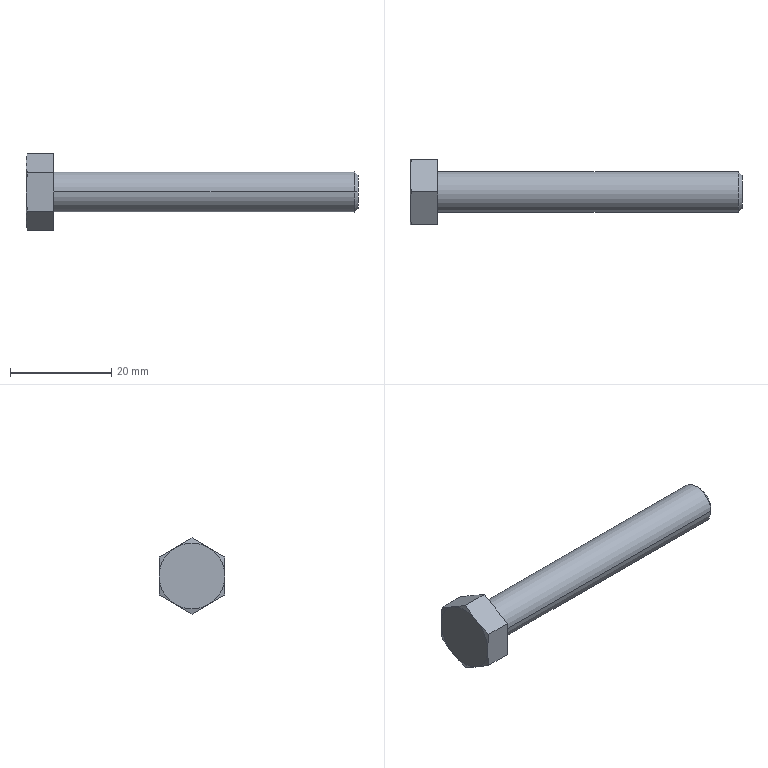Part | STEP file | TNSN20-Y20-F22-Part-1-1 | 1 solid | 19 faces | box 65.5 x 13.002 x 15.011 mm | volume 3813 mm3 | plane 9 | cone 8 | cylinder 2 | commonest cylinder face diameters 8 x2
STEP:
#1=CARTESIAN_POINT('',(13990.745,13720.046,26.506));
#2=VERTEX_POINT('',#1);
#3=CARTESIAN_POINT('',(13990.745,13713.546,22.753));
#4=VERTEX_POINT('',#3);
#5=CARTESIAN_POINT('',(13990.745,13720.046,26.506));
#6=DIRECTION('',(0.,-0.866,-0.5));
#7=VECTOR('',#6,1000.);
#8=LINE('',#5,#7);
#9=EDGE_CURVE('',#2,#4,#8,.T.);
#10=ORIENTED_EDGE('',*,*,#9,.T.);
#11=CARTESIAN_POINT('',(13990.745,13713.546,15.247));
#12=VERTEX_POINT('',#11);
#13=CARTESIAN_POINT('',(13990.745,13713.546,22.753));
#14=DIRECTION('',(0.,0.,-1.));
#15=VECTOR('',#14,1000.);
#16=LINE('',#13,#15);
#17=EDGE_CURVE('',#4,#12,#16,.T.);
#18=ORIENTED_EDGE('',*,*,#17,.T.);
#19=CARTESIAN_POINT('',(13990.745,13720.046,11.494));
#20=VERTEX_POINT('',#19);
#21=CARTESIAN_POINT('',(13990.745,13713.546,15.247));
#22=DIRECTION('',(0.,0.866,-0.5));
#23=VECTOR('',#22,1000.);
#24=LINE('',#21,#23);
#25=EDGE_CURVE('',#12,#20,#24,.T.);
#26=ORIENTED_EDGE('',*,*,#25,.T.);
#27=CARTESIAN_POINT('',(13990.745,13726.546,15.247));
#28=VERTEX_POINT('',#27);
#29=CARTESIAN_POINT('',(13990.745,13720.046,11.494));
#30=DIRECTION('',(0.,0.866,0.5));
#31=VECTOR('',#30,1000.);
#32=LINE('',#29,#31);
#33=EDGE_CURVE('',#20,#28,#32,.T.);
#34=ORIENTED_EDGE('',*,*,#33,.T.);
#35=CARTESIAN_POINT('',(13990.745,13726.546,22.753));
#36=VERTEX_POINT('',#35);
#37=CARTESIAN_POINT('',(13990.745,13726.546,15.247));
#38=DIRECTION('',(0.,0.,1.));
#39=VECTOR('',#38,1000.);
#40=LINE('',#37,#39);
#41=EDGE_CURVE('',#28,#36,#40,.T.);
#42=ORIENTED_EDGE('',*,*,#41,.T.);
#43=CARTESIAN_POINT('',(13990.745,13726.546,22.753));
#44=DIRECTION('',(0.,-0.866,0.5));
#45=VECTOR('',#44,1000.);
#46=LINE('',#43,#45);
#47=EDGE_CURVE('',#36,#2,#46,.T.);
#48=ORIENTED_EDGE('',*,*,#47,.T.);
#49=EDGE_LOOP('',(#10,#18,#26,#34,#42,#48));
#50=FACE_OUTER_BOUND('',#49,.T.);
#51=CARTESIAN_POINT('',(13990.745,13716.046,19.));
#52=VERTEX_POINT('',#51);
#53=CARTESIAN_POINT('',(13990.745,13724.046,19.));
#54=VERTEX_POINT('',#53);
#55=CARTESIAN_POINT('',(13990.745,13720.046,19.));
#56=DIRECTION('',(1.,0.,0.));
#57=DIRECTION('',(0.,1.,0.));
#58=AXIS2_PLACEMENT_3D('',#55,#56,#57);
#59=CIRCLE('',#58,4.);
#60=EDGE_CURVE('',#52,#54,#59,.T.);
#61=ORIENTED_EDGE('',*,*,#60,.F.);
#62=CARTESIAN_POINT('',(13990.745,13720.046,19.));
#63=DIRECTION('',(1.,0.,0.));
#64=DIRECTION('',(0.,1.,0.));
#65=AXIS2_PLACEMENT_3D('',#62,#63,#64);
#66=CIRCLE('',#65,4.);
#67=EDGE_CURVE('',#54,#52,#66,.T.);
#68=ORIENTED_EDGE('',*,*,#67,.F.);
#69=EDGE_LOOP('',(#61,#68));
#70=FACE_BOUND('',#69,.T.);
#71=CARTESIAN_POINT('',(13990.745,13734.949,3.347));
#72=DIRECTION('',(-1.,0.,0.));
#73=DIRECTION('',(0.,-1.,0.));
#74=AXIS2_PLACEMENT_3D('',#71,#72,#73);
#75=PLANE('',#74);
#76=ADVANCED_FACE('',(#50,#70),#75,.F.);
#77=CARTESIAN_POINT('',(14050.745,13723.279,19.));
#78=VERTEX_POINT('',#77);
#79=CARTESIAN_POINT('',(14050.745,13716.813,19.));
#80=VERTEX_POINT('',#79);
#81=CARTESIAN_POINT('',(14050.745,13720.046,19.));
#82=DIRECTION('',(1.,0.,0.));
#83=DIRECTION('',(0.,1.,0.));
#84=AXIS2_PLACEMENT_3D('',#81,#82,#83);
#85=CIRCLE('',#84,3.233);
#86=EDGE_CURVE('',#78,#80,#85,.T.);
#87=ORIENTED_EDGE('',*,*,#86,.T.);
#88=CARTESIAN_POINT('',(14050.745,13720.046,19.));
#89=DIRECTION('',(1.,0.,0.));
#90=DIRECTION('',(0.,1.,0.));
#91=AXIS2_PLACEMENT_3D('',#88,#89,#90);
#92=CIRCLE('',#91,3.233);
#93=EDGE_CURVE('',#80,#78,#92,.T.);
#94=ORIENTED_EDGE('',*,*,#93,.T.);
#95=EDGE_LOOP('',(#87,#94));
#96=FACE_OUTER_BOUND('',#95,.T.);
#97=CARTESIAN_POINT('',(14050.745,13729.541,7.888));
#98=DIRECTION('',(-1.,0.,0.));
#99=DIRECTION('',(0.,-1.,0.));
#100=AXIS2_PLACEMENT_3D('',#97,#98,#99);
#101=PLANE('',#100);
#102=ADVANCED_FACE('',(#96),#101,.F.);
#103=CARTESIAN_POINT('',(13985.514,13713.546,15.247));
#104=VERTEX_POINT('',#103);
#105=CARTESIAN_POINT('',(13990.745,13713.546,15.247));
#106=DIRECTION('',(-1.,0.,0.));
#107=VECTOR('',#106,1000.);
#108=LINE('',#105,#107);
#109=EDGE_CURVE('',#12,#104,#108,.T.);
#110=ORIENTED_EDGE('',*,*,#109,.F.);
#111=ORIENTED_EDGE('',*,*,#17,.F.);
#112=CARTESIAN_POINT('',(13985.514,13713.546,22.753));
#113=VERTEX_POINT('',#112);
#114=CARTESIAN_POINT('',(13990.745,13713.546,22.753));
#115=DIRECTION('',(-1.,0.,0.));
#116=VECTOR('',#115,1000.);
#117=LINE('',#114,#116);
#118=EDGE_CURVE('',#4,#113,#117,.T.);
#119=ORIENTED_EDGE('',*,*,#118,.T.);
#120=CARTESIAN_POINT('',(13985.245,13713.546,19.));
#121=VERTEX_POINT('',#120);
#122=CARTESIAN_POINT('',(13985.245,13713.546,19.));
#123=CARTESIAN_POINT('',(13985.244,13713.548,19.632));
#124=CARTESIAN_POINT('',(13985.27,13713.546,20.254));
#125=CARTESIAN_POINT('',(13985.363,13713.545,21.506));
#126=CARTESIAN_POINT('',(13985.431,13713.55,22.135));
#127=CARTESIAN_POINT('',(13985.514,13713.546,22.753));
#128=B_SPLINE_CURVE_WITH_KNOTS('',3,(#122,#123,#124,#125,#126,#127),.UNSPECIFIED.,.F.,.F.,(4,2,4),(0.,0.5,1.),.UNSPECIFIED.);
#129=EDGE_CURVE('',#121,#113,#128,.T.);
#130=ORIENTED_EDGE('',*,*,#129,.F.);
#131=CARTESIAN_POINT('',(13985.514,13713.546,15.247));
#132=CARTESIAN_POINT('',(13985.431,13713.55,15.865));
#133=CARTESIAN_POINT('',(13985.363,13713.546,16.494));
#134=CARTESIAN_POINT('',(13985.27,13713.546,17.746));
#135=CARTESIAN_POINT('',(13985.244,13713.548,18.368));
#136=CARTESIAN_POINT('',(13985.245,13713.546,19.));
#137=B_SPLINE_CURVE_WITH_KNOTS('',3,(#131,#132,#133,#134,#135,#136),.UNSPECIFIED.,.F.,.F.,(4,2,4),(0.,0.5,1.),.UNSPECIFIED.);
#138=EDGE_CURVE('',#104,#121,#137,.T.);
#139=ORIENTED_EDGE('',*,*,#138,.F.);
#140=EDGE_LOOP('',(#110,#111,#119,#130,#139));
#141=FACE_OUTER_BOUND('',#140,.T.);
#142=CARTESIAN_POINT('',(13994.974,13713.546,12.021));
#143=DIRECTION('',(0.,1.,0.));
#144=DIRECTION('',(-1.,0.,0.));
#145=AXIS2_PLACEMENT_3D('',#142,#143,#144);
#146=PLANE('',#145);
#147=ADVANCED_FACE('',(#141),#146,.F.);
#148=ORIENTED_EDGE('',*,*,#118,.F.);
#149=ORIENTED_EDGE('',*,*,#9,.F.);
#150=CARTESIAN_POINT('',(13985.514,13720.046,26.506));
#151=VERTEX_POINT('',#150);
#152=CARTESIAN_POINT('',(13990.745,13720.046,26.506));
#153=DIRECTION('',(-1.,0.,0.));
#154=VECTOR('',#153,1000.);
#155=LINE('',#152,#154);
#156=EDGE_CURVE('',#2,#151,#155,.T.);
#157=ORIENTED_EDGE('',*,*,#156,.T.);
#158=CARTESIAN_POINT('',(13985.245,13716.796,24.629));
#159=VERTEX_POINT('',#158);
#160=CARTESIAN_POINT('',(13985.245,13716.796,24.629));
#161=CARTESIAN_POINT('',(13985.244,13717.345,24.943));
#162=CARTESIAN_POINT('',(13985.27,13717.882,25.257));
#163=CARTESIAN_POINT('',(13985.363,13718.966,25.883));
#164=CARTESIAN_POINT('',(13985.431,13719.514,26.193));
#165=CARTESIAN_POINT('',(13985.514,13720.046,26.506));
#166=B_SPLINE_CURVE_WITH_KNOTS('',3,(#160,#161,#162,#163,#164,#165),.UNSPECIFIED.,.F.,.F.,(4,2,4),(0.,0.5,1.),.UNSPECIFIED.);
#167=EDGE_CURVE('',#159,#151,#166,.T.);
#168=ORIENTED_EDGE('',*,*,#167,.F.);
#169=CARTESIAN_POINT('',(13985.514,13713.546,22.753));
#170=CARTESIAN_POINT('',(13985.431,13714.083,23.058));
#171=CARTESIAN_POINT('',(13985.363,13714.626,23.377));
#172=CARTESIAN_POINT('',(13985.27,13715.71,24.003));
#173=CARTESIAN_POINT('',(13985.244,13716.25,24.311));
#174=CARTESIAN_POINT('',(13985.245,13716.796,24.629));
#175=B_SPLINE_CURVE_WITH_KNOTS('',3,(#169,#170,#171,#172,#173,#174),.UNSPECIFIED.,.F.,.F.,(4,2,4),(0.,0.5,1.),.UNSPECIFIED.);
#176=EDGE_CURVE('',#113,#159,#175,.T.);
#177=ORIENTED_EDGE('',*,*,#176,.F.);
#178=EDGE_LOOP('',(#148,#149,#157,#168,#177));
#179=FACE_OUTER_BOUND('',#178,.T.);
#180=CARTESIAN_POINT('',(13981.016,13710.753,21.14));
#181=DIRECTION('',(0.,0.5,-0.866));
#182=DIRECTION('',(0.,0.866,0.5));
#183=AXIS2_PLACEMENT_3D('',#180,#181,#182);
#184=PLANE('',#183);
#185=ADVANCED_FACE('',(#179),#184,.F.);
#186=ORIENTED_EDGE('',*,*,#156,.F.);
#187=ORIENTED_EDGE('',*,*,#47,.F.);
#188=CARTESIAN_POINT('',(13985.514,13726.546,22.753));
#189=VERTEX_POINT('',#188);
#190=CARTESIAN_POINT('',(13990.745,13726.546,22.753));
#191=DIRECTION('',(-1.,0.,0.));
#192=VECTOR('',#191,1000.);
#193=LINE('',#190,#192);
#194=EDGE_CURVE('',#36,#189,#193,.T.);
#195=ORIENTED_EDGE('',*,*,#194,.T.);
#196=CARTESIAN_POINT('',(13985.245,13723.296,24.629));
#197=VERTEX_POINT('',#196);
#198=CARTESIAN_POINT('',(13985.245,13723.296,24.629));
#199=CARTESIAN_POINT('',(13985.244,13723.843,24.311));
#200=CARTESIAN_POINT('',(13985.27,13724.383,24.003));
#201=CARTESIAN_POINT('',(13985.363,13725.467,23.377));
#202=CARTESIAN_POINT('',(13985.431,13726.01,23.058));
#203=CARTESIAN_POINT('',(13985.514,13726.546,22.753));
#204=B_SPLINE_CURVE_WITH_KNOTS('',3,(#198,#199,#200,#201,#202,#203),.UNSPECIFIED.,.F.,.F.,(4,2,4),(0.,0.5,1.),.UNSPECIFIED.);
#205=EDGE_CURVE('',#197,#189,#204,.T.);
#206=ORIENTED_EDGE('',*,*,#205,.F.);
#207=CARTESIAN_POINT('',(13985.514,13720.046,26.506));
#208=CARTESIAN_POINT('',(13985.431,13720.579,26.193));
#209=CARTESIAN_POINT('',(13985.363,13721.127,25.883));
#210=CARTESIAN_POINT('',(13985.27,13722.211,25.257));
#211=CARTESIAN_POINT('',(13985.244,13722.748,24.943));
#212=CARTESIAN_POINT('',(13985.245,13723.296,24.629));
#213=B_SPLINE_CURVE_WITH_KNOTS('',3,(#207,#208,#209,#210,#211,#212),.UNSPECIFIED.,.F.,.F.,(4,2,4),(0.,0.5,1.),.UNSPECIFIED.);
#214=EDGE_CURVE('',#151,#197,#213,.T.);
#215=ORIENTED_EDGE('',*,*,#214,.F.);
#216=EDGE_LOOP('',(#186,#187,#195,#206,#215));
#217=FACE_OUTER_BOUND('',#216,.T.);
#218=CARTESIAN_POINT('',(13981.016,13717.253,28.119));
#219=DIRECTION('',(0.,-0.5,-0.866));
#220=DIRECTION('',(0.,0.866,-0.5));
#221=AXIS2_PLACEMENT_3D('',#218,#219,#220);
#222=PLANE('',#221);
#223=ADVANCED_FACE('',(#217),#222,.F.);
#224=ORIENTED_EDGE('',*,*,#194,.F.);
#225=ORIENTED_EDGE('',*,*,#41,.F.);
#226=CARTESIAN_POINT('',(13985.514,13726.546,15.247));
#227=VERTEX_POINT('',#226);
#228=CARTESIAN_POINT('',(13990.745,13726.546,15.247));
#229=DIRECTION('',(-1.,0.,0.));
#230=VECTOR('',#229,1000.);
#231=LINE('',#228,#230);
#232=EDGE_CURVE('',#28,#227,#231,.T.);
#233=ORIENTED_EDGE('',*,*,#232,.T.);
#234=CARTESIAN_POINT('',(13985.245,13726.546,19.));
#235=VERTEX_POINT('',#234);
#236=CARTESIAN_POINT('',(13985.245,13726.546,19.));
#237=CARTESIAN_POINT('',(13985.244,13726.544,18.368));
#238=CARTESIAN_POINT('',(13985.27,13726.547,17.746));
#239=CARTESIAN_POINT('',(13985.363,13726.547,16.494));
#240=CARTESIAN_POINT('',(13985.431,13726.542,15.865));
#241=CARTESIAN_POINT('',(13985.514,13726.546,15.247));
#242=B_SPLINE_CURVE_WITH_KNOTS('',3,(#236,#237,#238,#239,#240,#241),.UNSPECIFIED.,.F.,.F.,(4,2,4),(0.,0.5,1.),.UNSPECIFIED.);
#243=EDGE_CURVE('',#235,#227,#242,.T.);
#244=ORIENTED_EDGE('',*,*,#243,.F.);
#245=CARTESIAN_POINT('',(13985.514,13726.546,22.753));
#246=CARTESIAN_POINT('',(13985.431,13726.542,22.135));
#247=CARTESIAN_POINT('',(13985.363,13726.547,21.506));
#248=CARTESIAN_POINT('',(13985.27,13726.547,20.254));
#249=CARTESIAN_POINT('',(13985.244,13726.544,19.632));
#250=CARTESIAN_POINT('',(13985.245,13726.546,19.));
#251=B_SPLINE_CURVE_WITH_KNOTS('',3,(#245,#246,#247,#248,#249,#250),.UNSPECIFIED.,.F.,.F.,(4,2,4),(0.,0.5,1.),.UNSPECIFIED.);
#252=EDGE_CURVE('',#189,#235,#251,.T.);
#253=ORIENTED_EDGE('',*,*,#252,.F.);
#254=EDGE_LOOP('',(#224,#225,#233,#244,#253));
#255=FACE_OUTER_BOUND('',#254,.T.);
#256=CARTESIAN_POINT('',(13981.016,13726.546,12.021));
#257=DIRECTION('',(0.,-1.,0.));
#258=DIRECTION('',(1.,0.,0.));
#259=AXIS2_PLACEMENT_3D('',#256,#257,#258);
#260=PLANE('',#259);
#261=ADVANCED_FACE('',(#255),#260,.F.);
#262=ORIENTED_EDGE('',*,*,#232,.F.);
#263=ORIENTED_EDGE('',*,*,#33,.F.);
#264=CARTESIAN_POINT('',(13985.514,13720.046,11.494));
#265=VERTEX_POINT('',#264);
#266=CARTESIAN_POINT('',(13990.745,13720.046,11.494));
#267=DIRECTION('',(-1.,0.,0.));
#268=VECTOR('',#267,1000.);
#269=LINE('',#266,#268);
#270=EDGE_CURVE('',#20,#265,#269,.T.);
#271=ORIENTED_EDGE('',*,*,#270,.T.);
#272=CARTESIAN_POINT('',(13985.245,13723.296,13.371));
#273=VERTEX_POINT('',#272);
#274=CARTESIAN_POINT('',(13985.245,13723.296,13.371));
#275=CARTESIAN_POINT('',(13985.244,13722.748,13.057));
#276=CARTESIAN_POINT('',(13985.27,13722.211,12.743));
#277=CARTESIAN_POINT('',(13985.363,13721.127,12.117));
#278=CARTESIAN_POINT('',(13985.431,13720.579,11.807));
#279=CARTESIAN_POINT('',(13985.514,13720.046,11.494));
#280=B_SPLINE_CURVE_WITH_KNOTS('',3,(#274,#275,#276,#277,#278,#279),.UNSPECIFIED.,.F.,.F.,(4,2,4),(0.,0.5,1.),.UNSPECIFIED.);
#281=EDGE_CURVE('',#273,#265,#280,.T.);
#282=ORIENTED_EDGE('',*,*,#281,.F.);
#283=CARTESIAN_POINT('',(13985.514,13726.546,15.247));
#284=CARTESIAN_POINT('',(13985.431,13726.01,14.942));
#285=CARTESIAN_POINT('',(13985.363,13725.467,14.623));
#286=CARTESIAN_POINT('',(13985.27,13724.383,13.997));
#287=CARTESIAN_POINT('',(13985.244,13723.843,13.689));
#288=CARTESIAN_POINT('',(13985.245,13723.296,13.371));
#289=B_SPLINE_CURVE_WITH_KNOTS('',3,(#283,#284,#285,#286,#287,#288),.UNSPECIFIED.,.F.,.F.,(4,2,4),(0.,0.5,1.),.UNSPECIFIED.);
#290=EDGE_CURVE('',#227,#273,#289,.T.);
#291=ORIENTED_EDGE('',*,*,#290,.F.);
#292=EDGE_LOOP('',(#262,#263,#271,#282,#291));
#293=FACE_OUTER_BOUND('',#292,.T.);
#294=CARTESIAN_POINT('',(13981.016,13729.34,16.86));
#295=DIRECTION('',(0.,-0.5,0.866));
#296=DIRECTION('',(0.,-0.866,-0.5));
#297=AXIS2_PLACEMENT_3D('',#294,#295,#296);
#298=PLANE('',#297);
#299=ADVANCED_FACE('',(#293),#298,.F.);
#300=ORIENTED_EDGE('',*,*,#270,.F.);
#301=ORIENTED_EDGE('',*,*,#25,.F.);
#302=ORIENTED_EDGE('',*,*,#109,.T.);
#303=CARTESIAN_POINT('',(13985.245,13716.796,13.371));
#304=VERTEX_POINT('',#303);
#305=CARTESIAN_POINT('',(13985.245,13716.796,13.371));
#306=CARTESIAN_POINT('',(13985.244,13716.25,13.689));
#307=CARTESIAN_POINT('',(13985.27,13715.71,13.997));
#308=CARTESIAN_POINT('',(13985.363,13714.626,14.623));
#309=CARTESIAN_POINT('',(13985.431,13714.083,14.942));
#310=CARTESIAN_POINT('',(13985.514,13713.546,15.247));
#311=B_SPLINE_CURVE_WITH_KNOTS('',3,(#305,#306,#307,#308,#309,#310),.UNSPECIFIED.,.F.,.F.,(4,2,4),(0.,0.5,1.),.UNSPECIFIED.);
#312=EDGE_CURVE('',#304,#104,#311,.T.);
#313=ORIENTED_EDGE('',*,*,#312,.F.);
#314=CARTESIAN_POINT('',(13985.514,13720.046,11.494));
#315=CARTESIAN_POINT('',(13985.431,13719.514,11.807));
#316=CARTESIAN_POINT('',(13985.363,13718.966,12.117));
#317=CARTESIAN_POINT('',(13985.27,13717.882,12.743));
#318=CARTESIAN_POINT('',(13985.244,13717.345,13.057));
#319=CARTESIAN_POINT('',(13985.245,13716.796,13.371));
#320=B_SPLINE_CURVE_WITH_KNOTS('',3,(#314,#315,#316,#317,#318,#319),.UNSPECIFIED.,.F.,.F.,(4,2,4),(0.,0.5,1.),.UNSPECIFIED.);
#321=EDGE_CURVE('',#265,#304,#320,.T.);
#322=ORIENTED_EDGE('',*,*,#321,.F.);
#323=EDGE_LOOP('',(#300,#301,#302,#313,#322));
#324=FACE_OUTER_BOUND('',#323,.T.);
#325=CARTESIAN_POINT('',(13981.016,13722.84,9.881));
#326=DIRECTION('',(0.,0.5,0.866));
#327=DIRECTION('',(0.,-0.866,0.5));
#328=AXIS2_PLACEMENT_3D('',#325,#326,#327);
#329=PLANE('',#328);
#330=ADVANCED_FACE('',(#324),#329,.F.);
#331=CARTESIAN_POINT('',(13985.245,13720.046,19.));
#332=DIRECTION('',(1.,0.,0.));
#333=DIRECTION('',(0.,-0.5,0.866));
#334=AXIS2_PLACEMENT_3D('',#331,#332,#333);
#335=CIRCLE('',#334,6.5);
#336=EDGE_CURVE('',#159,#121,#335,.T.);
#337=ORIENTED_EDGE('',*,*,#336,.T.);
#338=ORIENTED_EDGE('',*,*,#129,.T.);
#339=ORIENTED_EDGE('',*,*,#176,.T.);
#340=EDGE_LOOP('',(#337,#338,#339));
#341=FACE_OUTER_BOUND('',#340,.T.);
#342=CARTESIAN_POINT('',(13984.107,13720.046,19.));
#343=DIRECTION('',(1.,0.,0.));
#344=DIRECTION('',(0.,1.,0.));
#345=AXIS2_PLACEMENT_3D('',#342,#343,#344);
#346=CONICAL_SURFACE('',#345,2.253,1.309);
#347=ADVANCED_FACE('',(#341),#346,.T.);
#348=CARTESIAN_POINT('',(13985.245,13720.046,19.));
#349=DIRECTION('',(1.,0.,0.));
#350=DIRECTION('',(0.,-0.5,-0.866));
#351=AXIS2_PLACEMENT_3D('',#348,#349,#350);
#352=CIRCLE('',#351,6.5);
#353=EDGE_CURVE('',#304,#273,#352,.T.);
#354=ORIENTED_EDGE('',*,*,#353,.T.);
#355=ORIENTED_EDGE('',*,*,#281,.T.);
#356=ORIENTED_EDGE('',*,*,#321,.T.);
#357=EDGE_LOOP('',(#354,#355,#356));
#358=FACE_OUTER_BOUND('',#357,.T.);
#359=CARTESIAN_POINT('',(13984.055,13720.046,19.));
#360=DIRECTION('',(1.,0.,0.));
#361=DIRECTION('',(0.,1.,0.));
#362=AXIS2_PLACEMENT_3D('',#359,#360,#361);
#363=CONICAL_SURFACE('',#362,2.06,1.309);
#364=ADVANCED_FACE('',(#358),#363,.T.);
#365=CARTESIAN_POINT('',(13985.245,13720.046,19.));
#366=DIRECTION('',(1.,0.,0.));
#367=DIRECTION('',(0.,0.5,-0.866));
#368=AXIS2_PLACEMENT_3D('',#365,#366,#367);
#369=CIRCLE('',#368,6.5);
#370=EDGE_CURVE('',#273,#235,#369,.T.);
#371=ORIENTED_EDGE('',*,*,#370,.T.);
#372=ORIENTED_EDGE('',*,*,#243,.T.);
#373=ORIENTED_EDGE('',*,*,#290,.T.);
#374=EDGE_LOOP('',(#371,#372,#373));
#375=FACE_OUTER_BOUND('',#374,.T.);
#376=CARTESIAN_POINT('',(13984.107,13720.046,19.));
#377=DIRECTION('',(1.,0.,0.));
#378=DIRECTION('',(0.,-0.866,0.5));
#379=AXIS2_PLACEMENT_3D('',#376,#377,#378);
#380=CONICAL_SURFACE('',#379,2.253,1.309);
#381=ADVANCED_FACE('',(#375),#380,.T.);
#382=CARTESIAN_POINT('',(13985.245,13720.046,19.));
#383=DIRECTION('',(1.,0.,0.));
#384=DIRECTION('',(0.,1.,0.));
#385=AXIS2_PLACEMENT_3D('',#382,#383,#384);
#386=CIRCLE('',#385,6.5);
#387=EDGE_CURVE('',#235,#197,#386,.T.);
#388=ORIENTED_EDGE('',*,*,#387,.T.);
#389=ORIENTED_EDGE('',*,*,#205,.T.);
#390=ORIENTED_EDGE('',*,*,#252,.T.);
#391=EDGE_LOOP('',(#388,#389,#390));
#392=FACE_OUTER_BOUND('',#391,.T.);
#393=CARTESIAN_POINT('',(13984.107,13720.046,19.));
#394=DIRECTION('',(1.,0.,0.));
#395=DIRECTION('',(0.,-0.8704,-0.4924));
#396=AXIS2_PLACEMENT_3D('',#393,#394,#395);
#397=CONICAL_SURFACE('',#396,2.253,1.309);
#398=ADVANCED_FACE('',(#392),#397,.T.);
#399=ORIENTED_EDGE('',*,*,#214,.T.);
#400=CARTESIAN_POINT('',(13985.245,13720.046,19.));
#401=DIRECTION('',(1.,0.,0.));
#402=DIRECTION('',(0.,0.5,0.866));
#403=AXIS2_PLACEMENT_3D('',#400,#401,#402);
#404=CIRCLE('',#403,6.5);
#405=EDGE_CURVE('',#197,#159,#404,.T.);
#406=ORIENTED_EDGE('',*,*,#405,.T.);
#407=ORIENTED_EDGE('',*,*,#167,.T.);
#408=EDGE_LOOP('',(#399,#406,#407));
#409=FACE_OUTER_BOUND('',#408,.T.);
#410=CARTESIAN_POINT('',(13984.055,13720.046,19.));
#411=DIRECTION('',(1.,0.,0.));
#412=DIRECTION('',(0.,1.,0.));
#413=AXIS2_PLACEMENT_3D('',#410,#411,#412);
#414=CONICAL_SURFACE('',#413,2.06,1.309);
#415=ADVANCED_FACE('',(#409),#414,.T.);
#416=ORIENTED_EDGE('',*,*,#405,.F.);
#417=ORIENTED_EDGE('',*,*,#387,.F.);
#418=ORIENTED_EDGE('',*,*,#370,.F.);
#419=ORIENTED_EDGE('',*,*,#353,.F.);
#420=CARTESIAN_POINT('',(13985.245,13720.046,19.));
#421=DIRECTION('',(1.,0.,0.));
#422=DIRECTION('',(0.,-1.,0.));
#423=AXIS2_PLACEMENT_3D('',#420,#421,#422);
#424=CIRCLE('',#423,6.5);
#425=EDGE_CURVE('',#121,#304,#424,.T.);
#426=ORIENTED_EDGE('',*,*,#425,.F.);
#427=ORIENTED_EDGE('',*,*,#336,.F.);
#428=EDGE_LOOP('',(#416,#417,#418,#419,#426,#427));
#429=FACE_OUTER_BOUND('',#428,.T.);
#430=CARTESIAN_POINT('',(13985.245,13705.153,4.107));
#431=DIRECTION('',(1.,0.,0.));
#432=DIRECTION('',(0.,1.,0.));
#433=AXIS2_PLACEMENT_3D('',#430,#431,#432);
#434=PLANE('',#433);
#435=ADVANCED_FACE('',(#429),#434,.F.);
#436=ORIENTED_EDGE('',*,*,#312,.T.);
#437=ORIENTED_EDGE('',*,*,#138,.T.);
#438=ORIENTED_EDGE('',*,*,#425,.T.);
#439=EDGE_LOOP('',(#436,#437,#438));
#440=FACE_OUTER_BOUND('',#439,.T.);
#441=CARTESIAN_POINT('',(13984.107,13720.046,19.));
#442=DIRECTION('',(1.,0.,0.));
#443=DIRECTION('',(0.,1.,0.));
#444=AXIS2_PLACEMENT_3D('',#441,#442,#443);
#445=CONICAL_SURFACE('',#444,2.253,1.309);
#446=ADVANCED_FACE('',(#440),#445,.T.);
#447=CARTESIAN_POINT('',(14049.978,13716.046,19.));
#448=VERTEX_POINT('',#447);
#449=CARTESIAN_POINT('',(14049.978,13724.046,19.));
#450=VERTEX_POINT('',#449);
#451=CARTESIAN_POINT('',(14049.978,13720.046,19.));
#452=DIRECTION('',(1.,0.,0.));
#453=DIRECTION('',(0.,1.,0.));
#454=AXIS2_PLACEMENT_3D('',#451,#452,#453);
#455=CIRCLE('',#454,4.);
#456=EDGE_CURVE('',#448,#450,#455,.T.);
#457=ORIENTED_EDGE('',*,*,#456,.F.);
#458=CARTESIAN_POINT('',(13990.745,13716.046,19.));
#459=DIRECTION('',(1.,0.,0.));
#460=VECTOR('',#459,1000.);
#461=LINE('',#458,#460);
#462=EDGE_CURVE('',#52,#448,#461,.T.);
#463=ORIENTED_EDGE('',*,*,#462,.F.);
#464=ORIENTED_EDGE('',*,*,#60,.T.);
#465=CARTESIAN_POINT('',(13990.745,13724.046,19.));
#466=DIRECTION('',(1.,0.,0.));
#467=VECTOR('',#466,1000.);
#468=LINE('',#465,#467);
#469=EDGE_CURVE('',#54,#450,#468,.T.);
#470=ORIENTED_EDGE('',*,*,#469,.T.);
#471=EDGE_LOOP('',(#457,#463,#464,#470));
#472=FACE_OUTER_BOUND('',#471,.T.);
#473=CARTESIAN_POINT('',(14020.361,13720.046,19.));
#474=DIRECTION('',(1.,0.,0.));
#475=DIRECTION('',(0.,-1.,0.));
#476=AXIS2_PLACEMENT_3D('',#473,#474,#475);
#477=CYLINDRICAL_SURFACE('',#476,4.);
#478=ADVANCED_FACE('',(#472),#477,.T.);
#479=ORIENTED_EDGE('',*,*,#67,.T.);
#480=ORIENTED_EDGE('',*,*,#462,.T.);
#481=CARTESIAN_POINT('',(14049.978,13720.046,19.));
#482=DIRECTION('',(1.,0.,0.));
#483=DIRECTION('',(0.,1.,0.));
#484=AXIS2_PLACEMENT_3D('',#481,#482,#483);
#485=CIRCLE('',#484,4.);
#486=EDGE_CURVE('',#450,#448,#485,.T.);
#487=ORIENTED_EDGE('',*,*,#486,.F.);
#488=ORIENTED_EDGE('',*,*,#469,.F.);
#489=EDGE_LOOP('',(#479,#480,#487,#488));
#490=FACE_OUTER_BOUND('',#489,.T.);
#491=CARTESIAN_POINT('',(14020.361,13720.046,19.));
#492=DIRECTION('',(1.,0.,0.));
#493=DIRECTION('',(0.,-1.,0.));
#494=AXIS2_PLACEMENT_3D('',#491,#492,#493);
#495=CYLINDRICAL_SURFACE('',#494,4.);
#496=ADVANCED_FACE('',(#490),#495,.T.);
#497=ORIENTED_EDGE('',*,*,#93,.F.);
#498=CARTESIAN_POINT('',(14049.978,13716.046,19.));
#499=DIRECTION('',(0.7071,0.7071,0.));
#500=VECTOR('',#499,1000.);
#501=LINE('',#498,#500);
#502=EDGE_CURVE('',#448,#80,#501,.T.);
#503=ORIENTED_EDGE('',*,*,#502,.F.);
#504=ORIENTED_EDGE('',*,*,#456,.T.);
#505=CARTESIAN_POINT('',(14049.978,13724.046,19.));
#506=DIRECTION('',(0.7071,-0.7071,0.));
#507=VECTOR('',#506,1000.);
#508=LINE('',#505,#507);
#509=EDGE_CURVE('',#450,#78,#508,.T.);
#510=ORIENTED_EDGE('',*,*,#509,.T.);
#511=EDGE_LOOP('',(#497,#503,#504,#510));
#512=FACE_OUTER_BOUND('',#511,.T.);
#513=CARTESIAN_POINT('',(13053.978,13720.046,19.));
#514=DIRECTION('',(-1.,0.,0.));
#515=DIRECTION('',(0.,-1.,0.));
#516=AXIS2_PLACEMENT_3D('',#513,#514,#515);
#517=CONICAL_SURFACE('',#516,1000.,0.7854);
#518=ADVANCED_FACE('',(#512),#517,.T.);
#519=ORIENTED_EDGE('',*,*,#486,.T.);
#520=ORIENTED_EDGE('',*,*,#502,.T.);
#521=ORIENTED_EDGE('',*,*,#86,.F.);
#522=ORIENTED_EDGE('',*,*,#509,.F.);
#523=EDGE_LOOP('',(#519,#520,#521,#522));
#524=FACE_OUTER_BOUND('',#523,.T.);
#525=CARTESIAN_POINT('',(13053.978,13720.046,19.));
#526=DIRECTION('',(-1.,0.,0.));
#527=DIRECTION('',(0.,-1.,0.));
#528=AXIS2_PLACEMENT_3D('',#525,#526,#527);
#529=CONICAL_SURFACE('',#528,1000.,0.7854);
#530=ADVANCED_FACE('',(#524),#529,.T.);
#531=CLOSED_SHELL('',(#76,#102,#147,#185,#223,#261,#299,#330,#347,#364,#381,#398,#415,#435,#446,#478,#496,#518,#530));
#532=MANIFOLD_SOLID_BREP('',#531);
#533=CARTESIAN_POINT('',(0.,0.,0.));
#534=DIRECTION('',(0.,0.,1.));
#535=DIRECTION('',(1.,0.,0.));
#536=AXIS2_PLACEMENT_3D('',#533,#534,#535);
#537=(LENGTH_UNIT()NAMED_UNIT(*)SI_UNIT(.MILLI.,.METRE.));
#538=UNCERTAINTY_MEASURE_WITH_UNIT(LENGTH_MEASURE(0.00001),#537,'','');
#539=(NAMED_UNIT(*)PLANE_ANGLE_UNIT()SI_UNIT($,.RADIAN.));
#540=(NAMED_UNIT(*)SI_UNIT($,.STERADIAN.)SOLID_ANGLE_UNIT());
#541=(GEOMETRIC_REPRESENTATION_CONTEXT(3)GLOBAL_UNCERTAINTY_ASSIGNED_CONTEXT((#538))GLOBAL_UNIT_ASSIGNED_CONTEXT((#537,#539,#540))REPRESENTATION_CONTEXT('',''));
#542=ADVANCED_BREP_SHAPE_REPRESENTATION('',(#532,#536),#541);